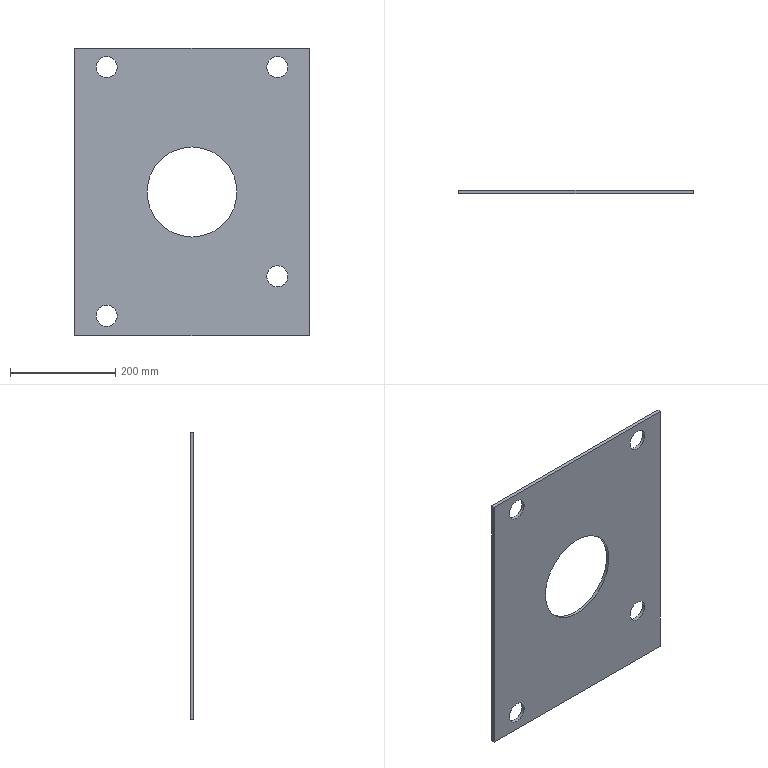Part | STEP file | INSULT-PLATE_id450_x_t | 1 solid | 11 faces | box 446 x 6 x 546 mm | volume 1293142 mm3 | plane 6 | cylinder 5 | commonest cylinder face diameters 40 x4 171 x1
STEP:
#1=CARTESIAN_POINT('',(162.,181.5,257.));
#2=VERTEX_POINT('',#1);
#3=CARTESIAN_POINT('',(162.,181.5,237.));
#4=DIRECTION('',(0.,-1.,0.));
#5=DIRECTION('',(0.,0.,1.));
#6=AXIS2_PLACEMENT_3D('',#3,#4,#5);
#7=CIRCLE('',#6,20.);
#8=EDGE_CURVE('',#2,#2,#7,.T.);
#9=ORIENTED_EDGE('',*,*,#8,.T.);
#10=EDGE_LOOP('',(#9));
#11=FACE_BOUND('',#10,.T.);
#12=CARTESIAN_POINT('',(-162.,181.5,257.));
#13=VERTEX_POINT('',#12);
#14=CARTESIAN_POINT('',(-162.,181.5,237.));
#15=DIRECTION('',(0.,-1.,0.));
#16=DIRECTION('',(0.,0.,1.));
#17=AXIS2_PLACEMENT_3D('',#14,#15,#16);
#18=CIRCLE('',#17,20.);
#19=EDGE_CURVE('',#13,#13,#18,.T.);
#20=ORIENTED_EDGE('',*,*,#19,.T.);
#21=EDGE_LOOP('',(#20));
#22=FACE_BOUND('',#21,.T.);
#23=CARTESIAN_POINT('',(-162.,181.5,-215.));
#24=VERTEX_POINT('',#23);
#25=CARTESIAN_POINT('',(-162.,181.5,-235.));
#26=DIRECTION('',(0.,-1.,0.));
#27=DIRECTION('',(0.,0.,1.));
#28=AXIS2_PLACEMENT_3D('',#25,#26,#27);
#29=CIRCLE('',#28,20.);
#30=EDGE_CURVE('',#24,#24,#29,.T.);
#31=ORIENTED_EDGE('',*,*,#30,.T.);
#32=EDGE_LOOP('',(#31));
#33=FACE_BOUND('',#32,.T.);
#34=CARTESIAN_POINT('',(162.,181.5,-140.));
#35=VERTEX_POINT('',#34);
#36=CARTESIAN_POINT('',(162.,181.5,-160.));
#37=DIRECTION('',(0.,-1.,0.));
#38=DIRECTION('',(0.,0.,1.));
#39=AXIS2_PLACEMENT_3D('',#36,#37,#38);
#40=CIRCLE('',#39,20.);
#41=EDGE_CURVE('',#35,#35,#40,.T.);
#42=ORIENTED_EDGE('',*,*,#41,.T.);
#43=EDGE_LOOP('',(#42));
#44=FACE_BOUND('',#43,.T.);
#45=CARTESIAN_POINT('',(0.,181.5,85.5));
#46=VERTEX_POINT('',#45);
#47=CARTESIAN_POINT('',(0.,181.5,0.));
#48=DIRECTION('',(0.,-1.,0.));
#49=DIRECTION('',(0.,0.,1.));
#50=AXIS2_PLACEMENT_3D('',#47,#48,#49);
#51=CIRCLE('',#50,85.5);
#52=EDGE_CURVE('',#46,#46,#51,.T.);
#53=ORIENTED_EDGE('',*,*,#52,.T.);
#54=EDGE_LOOP('',(#53));
#55=FACE_BOUND('',#54,.T.);
#56=CARTESIAN_POINT('',(-223.,181.5,-273.));
#57=VERTEX_POINT('',#56);
#58=CARTESIAN_POINT('',(223.,181.5,-273.));
#59=VERTEX_POINT('',#58);
#60=CARTESIAN_POINT('',(223.,181.5,-273.));
#61=DIRECTION('',(1.,0.,0.));
#62=VECTOR('',#61,1.);
#63=LINE('',#60,#62);
#64=EDGE_CURVE('',#57,#59,#63,.T.);
#65=ORIENTED_EDGE('',*,*,#64,.F.);
#66=CARTESIAN_POINT('',(-223.,181.5,273.));
#67=VERTEX_POINT('',#66);
#68=CARTESIAN_POINT('',(-223.,181.5,-273.));
#69=DIRECTION('',(0.,0.,-1.));
#70=VECTOR('',#69,1.);
#71=LINE('',#68,#70);
#72=EDGE_CURVE('',#67,#57,#71,.T.);
#73=ORIENTED_EDGE('',*,*,#72,.F.);
#74=CARTESIAN_POINT('',(223.,181.5,273.));
#75=VERTEX_POINT('',#74);
#76=CARTESIAN_POINT('',(-223.,181.5,273.));
#77=DIRECTION('',(-1.,0.,0.));
#78=VECTOR('',#77,1.);
#79=LINE('',#76,#78);
#80=EDGE_CURVE('',#75,#67,#79,.T.);
#81=ORIENTED_EDGE('',*,*,#80,.F.);
#82=CARTESIAN_POINT('',(223.,181.5,273.));
#83=DIRECTION('',(0.,0.,1.));
#84=VECTOR('',#83,1.);
#85=LINE('',#82,#84);
#86=EDGE_CURVE('',#59,#75,#85,.T.);
#87=ORIENTED_EDGE('',*,*,#86,.F.);
#88=EDGE_LOOP('',(#65,#73,#81,#87));
#89=FACE_BOUND('',#88,.T.);
#90=CARTESIAN_POINT('',(-200.,181.5,-275.));
#91=DIRECTION('',(0.,1.,0.));
#92=DIRECTION('',(0.,0.,1.));
#93=AXIS2_PLACEMENT_3D('',#90,#91,#92);
#94=PLANE('',#93);
#95=ADVANCED_FACE('',(#11,#22,#33,#44,#55,#89),#94,.T.);
#96=CARTESIAN_POINT('',(-223.,175.5,-273.));
#97=VERTEX_POINT('',#96);
#98=CARTESIAN_POINT('',(-223.,175.5,-273.));
#99=DIRECTION('',(0.,1.,0.));
#100=VECTOR('',#99,1.);
#101=LINE('',#98,#100);
#102=EDGE_CURVE('',#97,#57,#101,.T.);
#103=ORIENTED_EDGE('',*,*,#102,.F.);
#104=CARTESIAN_POINT('',(-223.,175.5,273.));
#105=VERTEX_POINT('',#104);
#106=CARTESIAN_POINT('',(-223.,175.5,-275.));
#107=DIRECTION('',(0.,0.,1.));
#108=VECTOR('',#107,1.);
#109=LINE('',#106,#108);
#110=EDGE_CURVE('',#97,#105,#109,.T.);
#111=ORIENTED_EDGE('',*,*,#110,.T.);
#112=CARTESIAN_POINT('',(-223.,175.5,273.));
#113=DIRECTION('',(0.,-1.,0.));
#114=VECTOR('',#113,1.);
#115=LINE('',#112,#114);
#116=EDGE_CURVE('',#67,#105,#115,.T.);
#117=ORIENTED_EDGE('',*,*,#116,.F.);
#118=ORIENTED_EDGE('',*,*,#72,.T.);
#119=EDGE_LOOP('',(#103,#111,#117,#118));
#120=FACE_OUTER_BOUND('',#119,.T.);
#121=CARTESIAN_POINT('',(-223.,175.5,-273.));
#122=DIRECTION('',(-1.,0.,0.));
#123=DIRECTION('',(0.,0.,1.));
#124=AXIS2_PLACEMENT_3D('',#121,#122,#123);
#125=PLANE('',#124);
#126=ADVANCED_FACE('',(#120),#125,.T.);
#127=ORIENTED_EDGE('',*,*,#116,.T.);
#128=CARTESIAN_POINT('',(223.,175.5,273.));
#129=VERTEX_POINT('',#128);
#130=CARTESIAN_POINT('',(-200.,175.5,273.));
#131=DIRECTION('',(1.,0.,0.));
#132=VECTOR('',#131,1.);
#133=LINE('',#130,#132);
#134=EDGE_CURVE('',#105,#129,#133,.T.);
#135=ORIENTED_EDGE('',*,*,#134,.T.);
#136=CARTESIAN_POINT('',(223.,175.5,273.));
#137=DIRECTION('',(0.,-1.,0.));
#138=VECTOR('',#137,1.);
#139=LINE('',#136,#138);
#140=EDGE_CURVE('',#75,#129,#139,.T.);
#141=ORIENTED_EDGE('',*,*,#140,.F.);
#142=ORIENTED_EDGE('',*,*,#80,.T.);
#143=EDGE_LOOP('',(#127,#135,#141,#142));
#144=FACE_OUTER_BOUND('',#143,.T.);
#145=CARTESIAN_POINT('',(-223.,175.5,273.));
#146=DIRECTION('',(0.,0.,1.));
#147=DIRECTION('',(1.,0.,0.));
#148=AXIS2_PLACEMENT_3D('',#145,#146,#147);
#149=PLANE('',#148);
#150=ADVANCED_FACE('',(#144),#149,.T.);
#151=ORIENTED_EDGE('',*,*,#140,.T.);
#152=CARTESIAN_POINT('',(223.,175.5,-273.));
#153=VERTEX_POINT('',#152);
#154=CARTESIAN_POINT('',(223.,175.5,-275.));
#155=DIRECTION('',(0.,0.,-1.));
#156=VECTOR('',#155,1.);
#157=LINE('',#154,#156);
#158=EDGE_CURVE('',#129,#153,#157,.T.);
#159=ORIENTED_EDGE('',*,*,#158,.T.);
#160=CARTESIAN_POINT('',(223.,175.5,-273.));
#161=DIRECTION('',(0.,-1.,0.));
#162=VECTOR('',#161,1.);
#163=LINE('',#160,#162);
#164=EDGE_CURVE('',#59,#153,#163,.T.);
#165=ORIENTED_EDGE('',*,*,#164,.F.);
#166=ORIENTED_EDGE('',*,*,#86,.T.);
#167=EDGE_LOOP('',(#151,#159,#165,#166));
#168=FACE_OUTER_BOUND('',#167,.T.);
#169=CARTESIAN_POINT('',(223.,175.5,273.));
#170=DIRECTION('',(1.,0.,0.));
#171=DIRECTION('',(0.,0.,-1.));
#172=AXIS2_PLACEMENT_3D('',#169,#170,#171);
#173=PLANE('',#172);
#174=ADVANCED_FACE('',(#168),#173,.T.);
#175=ORIENTED_EDGE('',*,*,#164,.T.);
#176=CARTESIAN_POINT('',(-200.,175.5,-273.));
#177=DIRECTION('',(-1.,0.,0.));
#178=VECTOR('',#177,1.);
#179=LINE('',#176,#178);
#180=EDGE_CURVE('',#153,#97,#179,.T.);
#181=ORIENTED_EDGE('',*,*,#180,.T.);
#182=ORIENTED_EDGE('',*,*,#102,.T.);
#183=ORIENTED_EDGE('',*,*,#64,.T.);
#184=EDGE_LOOP('',(#175,#181,#182,#183));
#185=FACE_OUTER_BOUND('',#184,.T.);
#186=CARTESIAN_POINT('',(223.,175.5,-273.));
#187=DIRECTION('',(0.,0.,-1.));
#188=DIRECTION('',(-1.,0.,0.));
#189=AXIS2_PLACEMENT_3D('',#186,#187,#188);
#190=PLANE('',#189);
#191=ADVANCED_FACE('',(#185),#190,.T.);
#192=ORIENTED_EDGE('',*,*,#52,.F.);
#193=EDGE_LOOP('',(#192));
#194=FACE_BOUND('',#193,.T.);
#195=CARTESIAN_POINT('',(0.,175.5,85.5));
#196=VERTEX_POINT('',#195);
#197=CARTESIAN_POINT('',(0.,175.5,0.));
#198=DIRECTION('',(0.,-1.,0.));
#199=DIRECTION('',(0.,0.,1.));
#200=AXIS2_PLACEMENT_3D('',#197,#198,#199);
#201=CIRCLE('',#200,85.5);
#202=EDGE_CURVE('',#196,#196,#201,.T.);
#203=ORIENTED_EDGE('',*,*,#202,.T.);
#204=EDGE_LOOP('',(#203));
#205=FACE_BOUND('',#204,.T.);
#206=CARTESIAN_POINT('',(0.,175.5,0.));
#207=DIRECTION('',(0.,1.,0.));
#208=DIRECTION('',(0.,0.,1.));
#209=AXIS2_PLACEMENT_3D('',#206,#207,#208);
#210=CYLINDRICAL_SURFACE('',#209,85.5);
#211=ADVANCED_FACE('',(#194,#205),#210,.F.);
#212=ORIENTED_EDGE('',*,*,#41,.F.);
#213=EDGE_LOOP('',(#212));
#214=FACE_BOUND('',#213,.T.);
#215=CARTESIAN_POINT('',(162.,175.5,-140.));
#216=VERTEX_POINT('',#215);
#217=CARTESIAN_POINT('',(162.,175.5,-160.));
#218=DIRECTION('',(0.,-1.,0.));
#219=DIRECTION('',(0.,0.,1.));
#220=AXIS2_PLACEMENT_3D('',#217,#218,#219);
#221=CIRCLE('',#220,20.);
#222=EDGE_CURVE('',#216,#216,#221,.T.);
#223=ORIENTED_EDGE('',*,*,#222,.T.);
#224=EDGE_LOOP('',(#223));
#225=FACE_BOUND('',#224,.T.);
#226=CARTESIAN_POINT('',(162.,181.5,-160.));
#227=DIRECTION('',(0.,1.,0.));
#228=DIRECTION('',(0.,0.,1.));
#229=AXIS2_PLACEMENT_3D('',#226,#227,#228);
#230=CYLINDRICAL_SURFACE('',#229,20.);
#231=ADVANCED_FACE('',(#214,#225),#230,.F.);
#232=ORIENTED_EDGE('',*,*,#30,.F.);
#233=EDGE_LOOP('',(#232));
#234=FACE_BOUND('',#233,.T.);
#235=CARTESIAN_POINT('',(-162.,175.5,-215.));
#236=VERTEX_POINT('',#235);
#237=CARTESIAN_POINT('',(-162.,175.5,-235.));
#238=DIRECTION('',(0.,-1.,0.));
#239=DIRECTION('',(0.,0.,1.));
#240=AXIS2_PLACEMENT_3D('',#237,#238,#239);
#241=CIRCLE('',#240,20.);
#242=EDGE_CURVE('',#236,#236,#241,.T.);
#243=ORIENTED_EDGE('',*,*,#242,.T.);
#244=EDGE_LOOP('',(#243));
#245=FACE_BOUND('',#244,.T.);
#246=CARTESIAN_POINT('',(-162.,181.5,-235.));
#247=DIRECTION('',(0.,1.,0.));
#248=DIRECTION('',(0.,0.,1.));
#249=AXIS2_PLACEMENT_3D('',#246,#247,#248);
#250=CYLINDRICAL_SURFACE('',#249,20.);
#251=ADVANCED_FACE('',(#234,#245),#250,.F.);
#252=ORIENTED_EDGE('',*,*,#19,.F.);
#253=EDGE_LOOP('',(#252));
#254=FACE_BOUND('',#253,.T.);
#255=CARTESIAN_POINT('',(-162.,175.5,257.));
#256=VERTEX_POINT('',#255);
#257=CARTESIAN_POINT('',(-162.,175.5,237.));
#258=DIRECTION('',(0.,-1.,0.));
#259=DIRECTION('',(0.,0.,1.));
#260=AXIS2_PLACEMENT_3D('',#257,#258,#259);
#261=CIRCLE('',#260,20.);
#262=EDGE_CURVE('',#256,#256,#261,.T.);
#263=ORIENTED_EDGE('',*,*,#262,.T.);
#264=EDGE_LOOP('',(#263));
#265=FACE_BOUND('',#264,.T.);
#266=CARTESIAN_POINT('',(-162.,181.5,237.));
#267=DIRECTION('',(0.,1.,0.));
#268=DIRECTION('',(0.,0.,1.));
#269=AXIS2_PLACEMENT_3D('',#266,#267,#268);
#270=CYLINDRICAL_SURFACE('',#269,20.);
#271=ADVANCED_FACE('',(#254,#265),#270,.F.);
#272=ORIENTED_EDGE('',*,*,#8,.F.);
#273=EDGE_LOOP('',(#272));
#274=FACE_BOUND('',#273,.T.);
#275=CARTESIAN_POINT('',(162.,175.5,257.));
#276=VERTEX_POINT('',#275);
#277=CARTESIAN_POINT('',(162.,175.5,237.));
#278=DIRECTION('',(0.,-1.,0.));
#279=DIRECTION('',(0.,0.,1.));
#280=AXIS2_PLACEMENT_3D('',#277,#278,#279);
#281=CIRCLE('',#280,20.);
#282=EDGE_CURVE('',#276,#276,#281,.T.);
#283=ORIENTED_EDGE('',*,*,#282,.T.);
#284=EDGE_LOOP('',(#283));
#285=FACE_BOUND('',#284,.T.);
#286=CARTESIAN_POINT('',(162.,181.5,237.));
#287=DIRECTION('',(0.,1.,0.));
#288=DIRECTION('',(0.,0.,1.));
#289=AXIS2_PLACEMENT_3D('',#286,#287,#288);
#290=CYLINDRICAL_SURFACE('',#289,20.);
#291=ADVANCED_FACE('',(#274,#285),#290,.F.);
#292=ORIENTED_EDGE('',*,*,#282,.F.);
#293=EDGE_LOOP('',(#292));
#294=FACE_BOUND('',#293,.T.);
#295=ORIENTED_EDGE('',*,*,#262,.F.);
#296=EDGE_LOOP('',(#295));
#297=FACE_BOUND('',#296,.T.);
#298=ORIENTED_EDGE('',*,*,#242,.F.);
#299=EDGE_LOOP('',(#298));
#300=FACE_BOUND('',#299,.T.);
#301=ORIENTED_EDGE('',*,*,#222,.F.);
#302=EDGE_LOOP('',(#301));
#303=FACE_BOUND('',#302,.T.);
#304=ORIENTED_EDGE('',*,*,#202,.F.);
#305=EDGE_LOOP('',(#304));
#306=FACE_BOUND('',#305,.T.);
#307=ORIENTED_EDGE('',*,*,#158,.F.);
#308=ORIENTED_EDGE('',*,*,#134,.F.);
#309=ORIENTED_EDGE('',*,*,#110,.F.);
#310=ORIENTED_EDGE('',*,*,#180,.F.);
#311=EDGE_LOOP('',(#307,#308,#309,#310));
#312=FACE_BOUND('',#311,.T.);
#313=CARTESIAN_POINT('',(-200.,175.5,-275.));
#314=DIRECTION('',(0.,1.,0.));
#315=DIRECTION('',(0.,0.,1.));
#316=AXIS2_PLACEMENT_3D('',#313,#314,#315);
#317=PLANE('',#316);
#318=ADVANCED_FACE('',(#294,#297,#300,#303,#306,#312),#317,.F.);
#319=CLOSED_SHELL('',(#95,#126,#150,#174,#191,#211,#231,#251,#271,#291,#318));
#320=MANIFOLD_SOLID_BREP('',#319);
#321=(LENGTH_UNIT()NAMED_UNIT(*)SI_UNIT(.MILLI.,.METRE.));
#322=UNCERTAINTY_MEASURE_WITH_UNIT(LENGTH_MEASURE(0.00002),#321,'','');
#323=(NAMED_UNIT(*)PLANE_ANGLE_UNIT()SI_UNIT($,.RADIAN.));
#324=PLANE_ANGLE_MEASURE_WITH_UNIT(PLANE_ANGLE_MEASURE(0.01745),#323);
#325=DIMENSIONAL_EXPONENTS(0.,0.,0.,0.,0.,0.,0.);
#326=(CONVERSION_BASED_UNIT('DEGREE',#324)NAMED_UNIT(#325)PLANE_ANGLE_UNIT());
#327=(NAMED_UNIT(*)SI_UNIT($,.STERADIAN.)SOLID_ANGLE_UNIT());
#328=(GEOMETRIC_REPRESENTATION_CONTEXT(3)GLOBAL_UNCERTAINTY_ASSIGNED_CONTEXT((#322))GLOBAL_UNIT_ASSIGNED_CONTEXT((#321,#326,#327))REPRESENTATION_CONTEXT('',''));
#329=ADVANCED_BREP_SHAPE_REPRESENTATION('',(#320),#328);